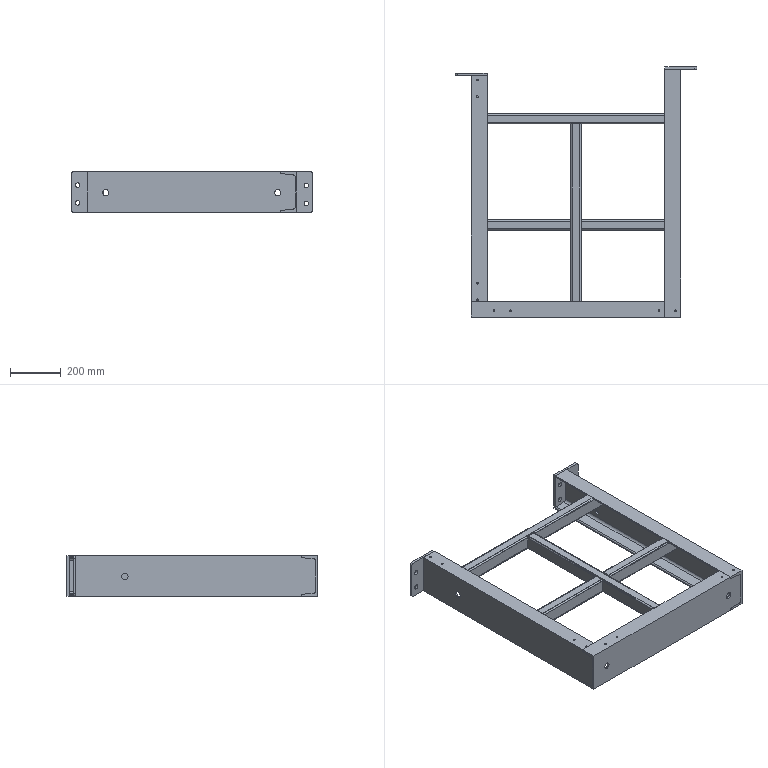Part | STEP file | PN_0052 steel stair platform 2_Default<As Machined> | 9 solids | 208 faces | box 951 x 986.002 x 160 mm | volume 7405397 mm3 | plane 110 | cylinder 97 | cone 1 | commonest cylinder face diameters 20 x20 6 x16 10 x16 12 x16 18 x16 6.8 x9